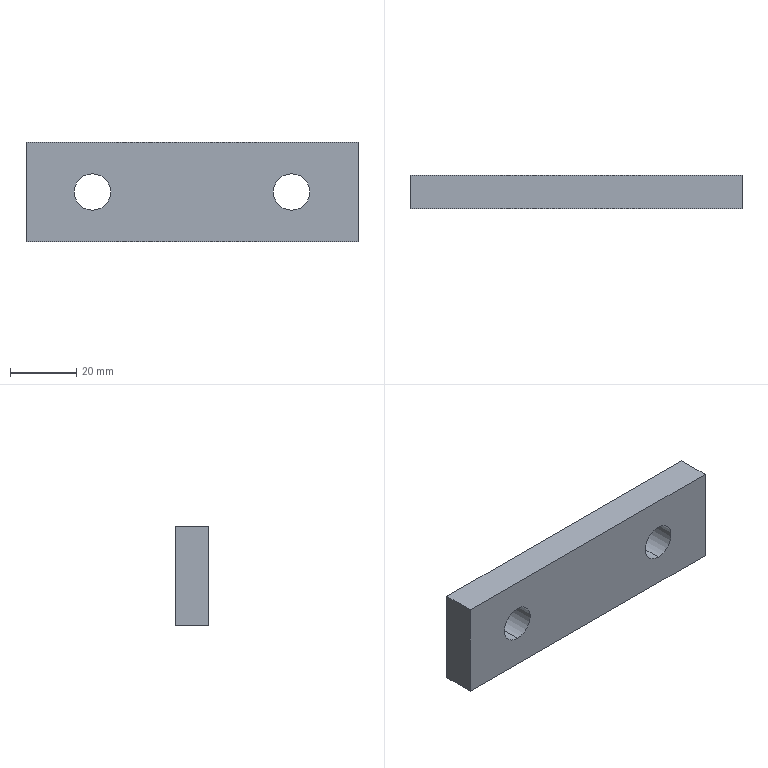Part | SolidWorks | features Extrusion 1, HoleWzd 1 | 1 solid | 10 faces | box 100 x 10 x 30 mm | volume 28099 mm3 | plane 6 | cylinder 4 | commonest cylinder face diameters 11 x4
STEP:
#1=CARTESIAN_POINT('',(-30.,0.,-5.5));
#2=VERTEX_POINT('',#1);
#3=CARTESIAN_POINT('',(-30.,0.,5.5));
#4=VERTEX_POINT('',#3);
#5=CARTESIAN_POINT('',(-30.,0.,0.));
#6=DIRECTION('',(0.,1.,0.));
#7=DIRECTION('',(0.,0.,1.));
#8=AXIS2_PLACEMENT_3D('',#5,#6,#7);
#9=CIRCLE('',#8,5.5);
#10=EDGE_CURVE('',#2,#4,#9,.T.);
#11=ORIENTED_EDGE('',*,*,#10,.F.);
#12=CARTESIAN_POINT('',(-30.,10.,-5.5));
#13=VERTEX_POINT('',#12);
#14=CARTESIAN_POINT('',(-30.,10.,-5.5));
#15=DIRECTION('',(0.,1.,0.));
#16=VECTOR('',#15,1000.);
#17=LINE('',#14,#16);
#18=EDGE_CURVE('',#2,#13,#17,.T.);
#19=ORIENTED_EDGE('',*,*,#18,.T.);
#20=CARTESIAN_POINT('',(-30.,10.,5.5));
#21=VERTEX_POINT('',#20);
#22=CARTESIAN_POINT('',(-30.,10.,0.));
#23=DIRECTION('',(0.,1.,0.));
#24=DIRECTION('',(0.,0.,1.));
#25=AXIS2_PLACEMENT_3D('',#22,#23,#24);
#26=CIRCLE('',#25,5.5);
#27=EDGE_CURVE('',#13,#21,#26,.T.);
#28=ORIENTED_EDGE('',*,*,#27,.T.);
#29=CARTESIAN_POINT('',(-30.,10.,5.5));
#30=DIRECTION('',(0.,1.,0.));
#31=VECTOR('',#30,1000.);
#32=LINE('',#29,#31);
#33=EDGE_CURVE('',#4,#21,#32,.T.);
#34=ORIENTED_EDGE('',*,*,#33,.F.);
#35=EDGE_LOOP('',(#11,#19,#28,#34));
#36=FACE_OUTER_BOUND('',#35,.T.);
#37=CARTESIAN_POINT('',(-30.,10.,0.));
#38=DIRECTION('',(0.,1.,0.));
#39=DIRECTION('',(0.,0.,1.));
#40=AXIS2_PLACEMENT_3D('',#37,#38,#39);
#41=CYLINDRICAL_SURFACE('',#40,5.5);
#42=ADVANCED_FACE('',(#36),#41,.F.);
#43=CARTESIAN_POINT('',(30.,0.,-5.5));
#44=VERTEX_POINT('',#43);
#45=CARTESIAN_POINT('',(30.,0.,5.5));
#46=VERTEX_POINT('',#45);
#47=CARTESIAN_POINT('',(30.,0.,0.));
#48=DIRECTION('',(0.,1.,0.));
#49=DIRECTION('',(0.,0.,1.));
#50=AXIS2_PLACEMENT_3D('',#47,#48,#49);
#51=CIRCLE('',#50,5.5);
#52=EDGE_CURVE('',#44,#46,#51,.T.);
#53=ORIENTED_EDGE('',*,*,#52,.F.);
#54=CARTESIAN_POINT('',(30.,10.,-5.5));
#55=VERTEX_POINT('',#54);
#56=CARTESIAN_POINT('',(30.,10.,-5.5));
#57=DIRECTION('',(0.,1.,0.));
#58=VECTOR('',#57,1000.);
#59=LINE('',#56,#58);
#60=EDGE_CURVE('',#44,#55,#59,.T.);
#61=ORIENTED_EDGE('',*,*,#60,.T.);
#62=CARTESIAN_POINT('',(30.,10.,5.5));
#63=VERTEX_POINT('',#62);
#64=CARTESIAN_POINT('',(30.,10.,0.));
#65=DIRECTION('',(0.,1.,0.));
#66=DIRECTION('',(0.,0.,1.));
#67=AXIS2_PLACEMENT_3D('',#64,#65,#66);
#68=CIRCLE('',#67,5.5);
#69=EDGE_CURVE('',#55,#63,#68,.T.);
#70=ORIENTED_EDGE('',*,*,#69,.T.);
#71=CARTESIAN_POINT('',(30.,10.,5.5));
#72=DIRECTION('',(0.,1.,0.));
#73=VECTOR('',#72,1000.);
#74=LINE('',#71,#73);
#75=EDGE_CURVE('',#46,#63,#74,.T.);
#76=ORIENTED_EDGE('',*,*,#75,.F.);
#77=EDGE_LOOP('',(#53,#61,#70,#76));
#78=FACE_OUTER_BOUND('',#77,.T.);
#79=CARTESIAN_POINT('',(30.,10.,0.));
#80=DIRECTION('',(0.,1.,0.));
#81=DIRECTION('',(0.,0.,1.));
#82=AXIS2_PLACEMENT_3D('',#79,#80,#81);
#83=CYLINDRICAL_SURFACE('',#82,5.5);
#84=ADVANCED_FACE('',(#78),#83,.F.);
#85=CARTESIAN_POINT('',(-50.,0.,-15.));
#86=VERTEX_POINT('',#85);
#87=CARTESIAN_POINT('',(-50.,0.,15.));
#88=VERTEX_POINT('',#87);
#89=CARTESIAN_POINT('',(-50.,0.,15.));
#90=DIRECTION('',(0.,0.,1.));
#91=VECTOR('',#90,1000.);
#92=LINE('',#89,#91);
#93=EDGE_CURVE('',#86,#88,#92,.T.);
#94=ORIENTED_EDGE('',*,*,#93,.T.);
#95=CARTESIAN_POINT('',(-50.,10.,15.));
#96=VERTEX_POINT('',#95);
#97=CARTESIAN_POINT('',(-50.,10.,15.));
#98=DIRECTION('',(0.,-1.,0.));
#99=VECTOR('',#98,1000.);
#100=LINE('',#97,#99);
#101=EDGE_CURVE('',#96,#88,#100,.T.);
#102=ORIENTED_EDGE('',*,*,#101,.F.);
#103=CARTESIAN_POINT('',(-50.,10.,-15.));
#104=VERTEX_POINT('',#103);
#105=CARTESIAN_POINT('',(-50.,10.,15.));
#106=DIRECTION('',(0.,0.,1.));
#107=VECTOR('',#106,1000.);
#108=LINE('',#105,#107);
#109=EDGE_CURVE('',#104,#96,#108,.T.);
#110=ORIENTED_EDGE('',*,*,#109,.F.);
#111=CARTESIAN_POINT('',(-50.,10.,-15.));
#112=DIRECTION('',(0.,-1.,0.));
#113=VECTOR('',#112,1000.);
#114=LINE('',#111,#113);
#115=EDGE_CURVE('',#104,#86,#114,.T.);
#116=ORIENTED_EDGE('',*,*,#115,.T.);
#117=EDGE_LOOP('',(#94,#102,#110,#116));
#118=FACE_OUTER_BOUND('',#117,.T.);
#119=CARTESIAN_POINT('',(-50.,10.,15.));
#120=DIRECTION('',(1.,0.,0.));
#121=DIRECTION('',(0.,0.,-1.));
#122=AXIS2_PLACEMENT_3D('',#119,#120,#121);
#123=PLANE('',#122);
#124=ADVANCED_FACE('',(#118),#123,.F.);
#125=CARTESIAN_POINT('',(50.,0.,15.));
#126=VERTEX_POINT('',#125);
#127=CARTESIAN_POINT('',(50.,0.,15.));
#128=DIRECTION('',(1.,0.,0.));
#129=VECTOR('',#128,1000.);
#130=LINE('',#127,#129);
#131=EDGE_CURVE('',#88,#126,#130,.T.);
#132=ORIENTED_EDGE('',*,*,#131,.T.);
#133=CARTESIAN_POINT('',(50.,10.,15.));
#134=VERTEX_POINT('',#133);
#135=CARTESIAN_POINT('',(50.,10.,15.));
#136=DIRECTION('',(0.,-1.,0.));
#137=VECTOR('',#136,1000.);
#138=LINE('',#135,#137);
#139=EDGE_CURVE('',#134,#126,#138,.T.);
#140=ORIENTED_EDGE('',*,*,#139,.F.);
#141=CARTESIAN_POINT('',(50.,10.,15.));
#142=DIRECTION('',(1.,0.,0.));
#143=VECTOR('',#142,1000.);
#144=LINE('',#141,#143);
#145=EDGE_CURVE('',#96,#134,#144,.T.);
#146=ORIENTED_EDGE('',*,*,#145,.F.);
#147=ORIENTED_EDGE('',*,*,#101,.T.);
#148=EDGE_LOOP('',(#132,#140,#146,#147));
#149=FACE_OUTER_BOUND('',#148,.T.);
#150=CARTESIAN_POINT('',(50.,10.,15.));
#151=DIRECTION('',(0.,0.,-1.));
#152=DIRECTION('',(-1.,0.,0.));
#153=AXIS2_PLACEMENT_3D('',#150,#151,#152);
#154=PLANE('',#153);
#155=ADVANCED_FACE('',(#149),#154,.F.);
#156=CARTESIAN_POINT('',(50.,0.,-15.));
#157=VERTEX_POINT('',#156);
#158=CARTESIAN_POINT('',(50.,0.,15.));
#159=DIRECTION('',(0.,0.,-1.));
#160=VECTOR('',#159,1000.);
#161=LINE('',#158,#160);
#162=EDGE_CURVE('',#126,#157,#161,.T.);
#163=ORIENTED_EDGE('',*,*,#162,.T.);
#164=CARTESIAN_POINT('',(50.,10.,-15.));
#165=VERTEX_POINT('',#164);
#166=CARTESIAN_POINT('',(50.,10.,-15.));
#167=DIRECTION('',(0.,-1.,0.));
#168=VECTOR('',#167,1000.);
#169=LINE('',#166,#168);
#170=EDGE_CURVE('',#165,#157,#169,.T.);
#171=ORIENTED_EDGE('',*,*,#170,.F.);
#172=CARTESIAN_POINT('',(50.,10.,15.));
#173=DIRECTION('',(0.,0.,-1.));
#174=VECTOR('',#173,1000.);
#175=LINE('',#172,#174);
#176=EDGE_CURVE('',#134,#165,#175,.T.);
#177=ORIENTED_EDGE('',*,*,#176,.F.);
#178=ORIENTED_EDGE('',*,*,#139,.T.);
#179=EDGE_LOOP('',(#163,#171,#177,#178));
#180=FACE_OUTER_BOUND('',#179,.T.);
#181=CARTESIAN_POINT('',(50.,10.,15.));
#182=DIRECTION('',(-1.,0.,0.));
#183=DIRECTION('',(0.,0.,1.));
#184=AXIS2_PLACEMENT_3D('',#181,#182,#183);
#185=PLANE('',#184);
#186=ADVANCED_FACE('',(#180),#185,.F.);
#187=CARTESIAN_POINT('',(50.,0.,-15.));
#188=DIRECTION('',(-1.,0.,0.));
#189=VECTOR('',#188,1000.);
#190=LINE('',#187,#189);
#191=EDGE_CURVE('',#157,#86,#190,.T.);
#192=ORIENTED_EDGE('',*,*,#191,.T.);
#193=ORIENTED_EDGE('',*,*,#115,.F.);
#194=CARTESIAN_POINT('',(50.,10.,-15.));
#195=DIRECTION('',(-1.,0.,0.));
#196=VECTOR('',#195,1000.);
#197=LINE('',#194,#196);
#198=EDGE_CURVE('',#165,#104,#197,.T.);
#199=ORIENTED_EDGE('',*,*,#198,.F.);
#200=ORIENTED_EDGE('',*,*,#170,.T.);
#201=EDGE_LOOP('',(#192,#193,#199,#200));
#202=FACE_OUTER_BOUND('',#201,.T.);
#203=CARTESIAN_POINT('',(50.,10.,-15.));
#204=DIRECTION('',(0.,0.,1.));
#205=DIRECTION('',(1.,0.,0.));
#206=AXIS2_PLACEMENT_3D('',#203,#204,#205);
#207=PLANE('',#206);
#208=ADVANCED_FACE('',(#202),#207,.F.);
#209=CARTESIAN_POINT('',(-30.,10.,0.));
#210=DIRECTION('',(0.,1.,0.));
#211=DIRECTION('',(0.,0.,1.));
#212=AXIS2_PLACEMENT_3D('',#209,#210,#211);
#213=CIRCLE('',#212,5.5);
#214=EDGE_CURVE('',#21,#13,#213,.T.);
#215=ORIENTED_EDGE('',*,*,#214,.F.);
#216=ORIENTED_EDGE('',*,*,#27,.F.);
#217=EDGE_LOOP('',(#215,#216));
#218=FACE_BOUND('',#217,.T.);
#219=CARTESIAN_POINT('',(30.,10.,0.));
#220=DIRECTION('',(0.,1.,0.));
#221=DIRECTION('',(0.,0.,1.));
#222=AXIS2_PLACEMENT_3D('',#219,#220,#221);
#223=CIRCLE('',#222,5.5);
#224=EDGE_CURVE('',#63,#55,#223,.T.);
#225=ORIENTED_EDGE('',*,*,#224,.F.);
#226=ORIENTED_EDGE('',*,*,#69,.F.);
#227=EDGE_LOOP('',(#225,#226));
#228=FACE_BOUND('',#227,.T.);
#229=ORIENTED_EDGE('',*,*,#109,.T.);
#230=ORIENTED_EDGE('',*,*,#145,.T.);
#231=ORIENTED_EDGE('',*,*,#176,.T.);
#232=ORIENTED_EDGE('',*,*,#198,.T.);
#233=EDGE_LOOP('',(#229,#230,#231,#232));
#234=FACE_OUTER_BOUND('',#233,.T.);
#235=CARTESIAN_POINT('',(0.,10.,0.));
#236=DIRECTION('',(0.,1.,0.));
#237=DIRECTION('',(0.,0.,1.));
#238=AXIS2_PLACEMENT_3D('',#235,#236,#237);
#239=PLANE('',#238);
#240=ADVANCED_FACE('',(#218,#228,#234),#239,.T.);
#241=CARTESIAN_POINT('',(-30.,0.,0.));
#242=DIRECTION('',(0.,1.,0.));
#243=DIRECTION('',(0.,0.,1.));
#244=AXIS2_PLACEMENT_3D('',#241,#242,#243);
#245=CIRCLE('',#244,5.5);
#246=EDGE_CURVE('',#4,#2,#245,.T.);
#247=ORIENTED_EDGE('',*,*,#246,.T.);
#248=ORIENTED_EDGE('',*,*,#10,.T.);
#249=EDGE_LOOP('',(#247,#248));
#250=FACE_BOUND('',#249,.T.);
#251=CARTESIAN_POINT('',(30.,0.,0.));
#252=DIRECTION('',(0.,1.,0.));
#253=DIRECTION('',(0.,0.,1.));
#254=AXIS2_PLACEMENT_3D('',#251,#252,#253);
#255=CIRCLE('',#254,5.5);
#256=EDGE_CURVE('',#46,#44,#255,.T.);
#257=ORIENTED_EDGE('',*,*,#256,.T.);
#258=ORIENTED_EDGE('',*,*,#52,.T.);
#259=EDGE_LOOP('',(#257,#258));
#260=FACE_BOUND('',#259,.T.);
#261=ORIENTED_EDGE('',*,*,#93,.F.);
#262=ORIENTED_EDGE('',*,*,#191,.F.);
#263=ORIENTED_EDGE('',*,*,#162,.F.);
#264=ORIENTED_EDGE('',*,*,#131,.F.);
#265=EDGE_LOOP('',(#261,#262,#263,#264));
#266=FACE_OUTER_BOUND('',#265,.T.);
#267=CARTESIAN_POINT('',(0.,0.,0.));
#268=DIRECTION('',(0.,1.,0.));
#269=DIRECTION('',(0.,0.,1.));
#270=AXIS2_PLACEMENT_3D('',#267,#268,#269);
#271=PLANE('',#270);
#272=ADVANCED_FACE('',(#250,#260,#266),#271,.F.);
#273=ORIENTED_EDGE('',*,*,#60,.F.);
#274=ORIENTED_EDGE('',*,*,#256,.F.);
#275=ORIENTED_EDGE('',*,*,#75,.T.);
#276=ORIENTED_EDGE('',*,*,#224,.T.);
#277=EDGE_LOOP('',(#273,#274,#275,#276));
#278=FACE_OUTER_BOUND('',#277,.T.);
#279=CARTESIAN_POINT('',(30.,10.,0.));
#280=DIRECTION('',(0.,1.,0.));
#281=DIRECTION('',(0.,0.,1.));
#282=AXIS2_PLACEMENT_3D('',#279,#280,#281);
#283=CYLINDRICAL_SURFACE('',#282,5.5);
#284=ADVANCED_FACE('',(#278),#283,.F.);
#285=ORIENTED_EDGE('',*,*,#18,.F.);
#286=ORIENTED_EDGE('',*,*,#246,.F.);
#287=ORIENTED_EDGE('',*,*,#33,.T.);
#288=ORIENTED_EDGE('',*,*,#214,.T.);
#289=EDGE_LOOP('',(#285,#286,#287,#288));
#290=FACE_OUTER_BOUND('',#289,.T.);
#291=CARTESIAN_POINT('',(-30.,10.,0.));
#292=DIRECTION('',(0.,1.,0.));
#293=DIRECTION('',(0.,0.,1.));
#294=AXIS2_PLACEMENT_3D('',#291,#292,#293);
#295=CYLINDRICAL_SURFACE('',#294,5.5);
#296=ADVANCED_FACE('',(#290),#295,.F.);
#297=CLOSED_SHELL('',(#42,#84,#124,#155,#186,#208,#240,#272,#284,#296));
#298=MANIFOLD_SOLID_BREP('',#297);
#299=CARTESIAN_POINT('',(0.,0.,0.));
#300=DIRECTION('',(0.,0.,1.));
#301=DIRECTION('',(1.,0.,0.));
#302=AXIS2_PLACEMENT_3D('',#299,#300,#301);
#303=(LENGTH_UNIT()NAMED_UNIT(*)SI_UNIT(.MILLI.,.METRE.));
#304=UNCERTAINTY_MEASURE_WITH_UNIT(LENGTH_MEASURE(0.00001),#303,'','');
#305=(NAMED_UNIT(*)PLANE_ANGLE_UNIT()SI_UNIT($,.RADIAN.));
#306=(NAMED_UNIT(*)SI_UNIT($,.STERADIAN.)SOLID_ANGLE_UNIT());
#307=(GEOMETRIC_REPRESENTATION_CONTEXT(3)GLOBAL_UNCERTAINTY_ASSIGNED_CONTEXT((#304))GLOBAL_UNIT_ASSIGNED_CONTEXT((#303,#305,#306))REPRESENTATION_CONTEXT('',''));
#308=ADVANCED_BREP_SHAPE_REPRESENTATION('',(#298,#302),#307);